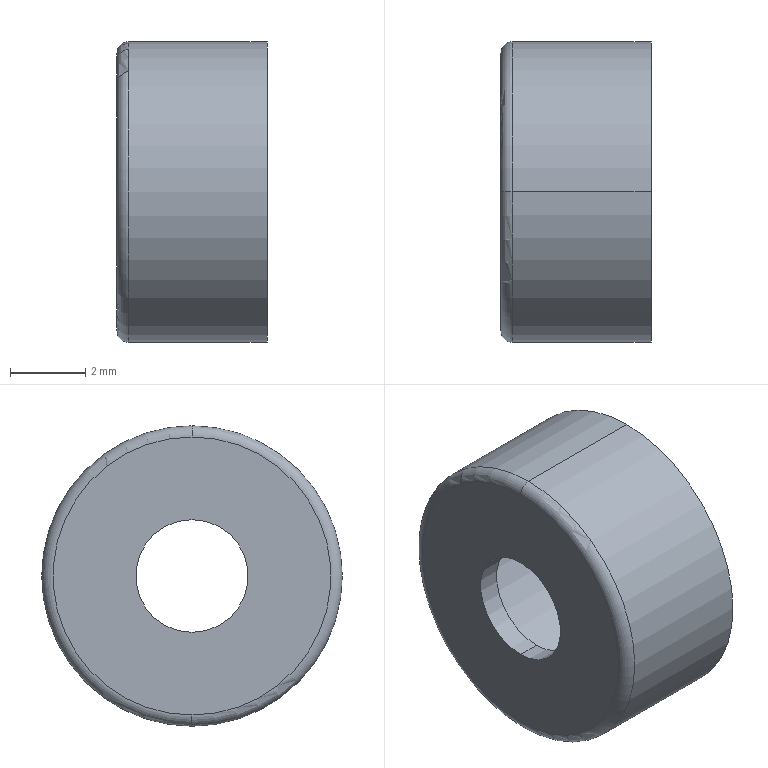Part | STEP file | 11-FG99-HXCC8b-V3.0-kkkkkk-998.11 | 1 solid | 11 faces | box 4 x 8 x 8 mm | volume 72.866 mm3 | cylinder 6 | plane 3 | torus 2 | commonest cylinder face diameters 3 x2 6.8 x2 8 x2
STEP:
#1=CARTESIAN_POINT('',(4.,0.,4.));
#2=VERTEX_POINT('',#1);
#3=CARTESIAN_POINT('',(4.,0.,-4.));
#4=VERTEX_POINT('',#3);
#5=CARTESIAN_POINT('',(4.,0.,0.));
#6=DIRECTION('',(-1.,0.,0.));
#7=DIRECTION('',(0.,0.,1.));
#8=AXIS2_PLACEMENT_3D('',#5,#6,#7);
#9=CIRCLE('',#8,4.);
#10=EDGE_CURVE('',#2,#4,#9,.T.);
#11=ORIENTED_EDGE('',*,*,#10,.T.);
#12=CARTESIAN_POINT('',(0.3,0.,-4.));
#13=VERTEX_POINT('',#12);
#14=CARTESIAN_POINT('',(4.,0.,-4.));
#15=DIRECTION('',(-1.,0.,0.));
#16=VECTOR('',#15,1000.);
#17=LINE('',#14,#16);
#18=EDGE_CURVE('',#4,#13,#17,.T.);
#19=ORIENTED_EDGE('',*,*,#18,.T.);
#20=CARTESIAN_POINT('',(0.3,0.,4.));
#21=VERTEX_POINT('',#20);
#22=CARTESIAN_POINT('',(0.3,0.,0.));
#23=DIRECTION('',(-1.,0.,0.));
#24=DIRECTION('',(0.,0.,1.));
#25=AXIS2_PLACEMENT_3D('',#22,#23,#24);
#26=CIRCLE('',#25,4.);
#27=EDGE_CURVE('',#21,#13,#26,.T.);
#28=ORIENTED_EDGE('',*,*,#27,.F.);
#29=CARTESIAN_POINT('',(4.,0.,4.));
#30=DIRECTION('',(-1.,0.,0.));
#31=VECTOR('',#30,1000.);
#32=LINE('',#29,#31);
#33=EDGE_CURVE('',#2,#21,#32,.T.);
#34=ORIENTED_EDGE('',*,*,#33,.F.);
#35=EDGE_LOOP('',(#11,#19,#28,#34));
#36=FACE_OUTER_BOUND('',#35,.T.);
#37=CARTESIAN_POINT('',(4.,0.,0.));
#38=DIRECTION('',(-1.,0.,0.));
#39=DIRECTION('',(0.,0.,1.));
#40=AXIS2_PLACEMENT_3D('',#37,#38,#39);
#41=CYLINDRICAL_SURFACE('',#40,4.);
#42=ADVANCED_FACE('',(#36),#41,.T.);
#43=CARTESIAN_POINT('',(4.,0.,-3.4));
#44=VERTEX_POINT('',#43);
#45=CARTESIAN_POINT('',(4.,0.,3.4));
#46=VERTEX_POINT('',#45);
#47=CARTESIAN_POINT('',(4.,0.,0.));
#48=DIRECTION('',(-1.,0.,0.));
#49=DIRECTION('',(0.,0.,1.));
#50=AXIS2_PLACEMENT_3D('',#47,#48,#49);
#51=CIRCLE('',#50,3.4);
#52=EDGE_CURVE('',#44,#46,#51,.T.);
#53=ORIENTED_EDGE('',*,*,#52,.F.);
#54=CARTESIAN_POINT('',(0.6,0.,-3.4));
#55=VERTEX_POINT('',#54);
#56=CARTESIAN_POINT('',(4.,0.,-3.4));
#57=DIRECTION('',(-1.,0.,0.));
#58=VECTOR('',#57,1000.);
#59=LINE('',#56,#58);
#60=EDGE_CURVE('',#44,#55,#59,.T.);
#61=ORIENTED_EDGE('',*,*,#60,.T.);
#62=CARTESIAN_POINT('',(0.6,0.,3.4));
#63=VERTEX_POINT('',#62);
#64=CARTESIAN_POINT('',(0.6,0.,0.));
#65=DIRECTION('',(-1.,0.,0.));
#66=DIRECTION('',(0.,0.,1.));
#67=AXIS2_PLACEMENT_3D('',#64,#65,#66);
#68=CIRCLE('',#67,3.4);
#69=EDGE_CURVE('',#55,#63,#68,.T.);
#70=ORIENTED_EDGE('',*,*,#69,.T.);
#71=CARTESIAN_POINT('',(4.,0.,3.4));
#72=DIRECTION('',(-1.,0.,0.));
#73=VECTOR('',#72,1000.);
#74=LINE('',#71,#73);
#75=EDGE_CURVE('',#46,#63,#74,.T.);
#76=ORIENTED_EDGE('',*,*,#75,.F.);
#77=EDGE_LOOP('',(#53,#61,#70,#76));
#78=FACE_OUTER_BOUND('',#77,.T.);
#79=CARTESIAN_POINT('',(4.,0.,0.));
#80=DIRECTION('',(-1.,0.,0.));
#81=DIRECTION('',(0.,0.,1.));
#82=AXIS2_PLACEMENT_3D('',#79,#80,#81);
#83=CYLINDRICAL_SURFACE('',#82,3.4);
#84=ADVANCED_FACE('',(#78),#83,.F.);
#85=CARTESIAN_POINT('',(0.6,0.,-1.5));
#86=VERTEX_POINT('',#85);
#87=CARTESIAN_POINT('',(0.6,0.,1.5));
#88=VERTEX_POINT('',#87);
#89=CARTESIAN_POINT('',(0.6,0.,0.));
#90=DIRECTION('',(-1.,0.,0.));
#91=DIRECTION('',(0.,0.,1.));
#92=AXIS2_PLACEMENT_3D('',#89,#90,#91);
#93=CIRCLE('',#92,1.5);
#94=EDGE_CURVE('',#86,#88,#93,.T.);
#95=ORIENTED_EDGE('',*,*,#94,.F.);
#96=CARTESIAN_POINT('',(0.,0.,-1.5));
#97=VERTEX_POINT('',#96);
#98=CARTESIAN_POINT('',(4.,0.,-1.5));
#99=DIRECTION('',(-1.,0.,0.));
#100=VECTOR('',#99,1000.);
#101=LINE('',#98,#100);
#102=EDGE_CURVE('',#86,#97,#101,.T.);
#103=ORIENTED_EDGE('',*,*,#102,.T.);
#104=CARTESIAN_POINT('',(0.,0.,1.5));
#105=VERTEX_POINT('',#104);
#106=CARTESIAN_POINT('',(0.,0.,0.));
#107=DIRECTION('',(-1.,0.,0.));
#108=DIRECTION('',(0.,0.,1.));
#109=AXIS2_PLACEMENT_3D('',#106,#107,#108);
#110=CIRCLE('',#109,1.5);
#111=EDGE_CURVE('',#97,#105,#110,.T.);
#112=ORIENTED_EDGE('',*,*,#111,.T.);
#113=CARTESIAN_POINT('',(4.,0.,1.5));
#114=DIRECTION('',(-1.,0.,0.));
#115=VECTOR('',#114,1000.);
#116=LINE('',#113,#115);
#117=EDGE_CURVE('',#88,#105,#116,.T.);
#118=ORIENTED_EDGE('',*,*,#117,.F.);
#119=EDGE_LOOP('',(#95,#103,#112,#118));
#120=FACE_OUTER_BOUND('',#119,.T.);
#121=CARTESIAN_POINT('',(4.,0.,0.));
#122=DIRECTION('',(-1.,0.,0.));
#123=DIRECTION('',(0.,0.,1.));
#124=AXIS2_PLACEMENT_3D('',#121,#122,#123);
#125=CYLINDRICAL_SURFACE('',#124,1.5);
#126=ADVANCED_FACE('',(#120),#125,.F.);
#127=ORIENTED_EDGE('',*,*,#27,.T.);
#128=CARTESIAN_POINT('',(0.,0.,-3.7));
#129=VERTEX_POINT('',#128);
#130=CARTESIAN_POINT('',(0.3,0.,-3.7));
#131=DIRECTION('',(0.,1.,0.));
#132=DIRECTION('',(0.,0.,1.));
#133=AXIS2_PLACEMENT_3D('',#130,#131,#132);
#134=CIRCLE('',#133,0.3);
#135=EDGE_CURVE('',#13,#129,#134,.T.);
#136=ORIENTED_EDGE('',*,*,#135,.T.);
#137=CARTESIAN_POINT('',(0.,0.,3.7));
#138=VERTEX_POINT('',#137);
#139=CARTESIAN_POINT('',(0.,0.,0.));
#140=DIRECTION('',(-1.,0.,0.));
#141=DIRECTION('',(0.,0.,1.));
#142=AXIS2_PLACEMENT_3D('',#139,#140,#141);
#143=CIRCLE('',#142,3.7);
#144=EDGE_CURVE('',#138,#129,#143,.T.);
#145=ORIENTED_EDGE('',*,*,#144,.F.);
#146=CARTESIAN_POINT('',(0.3,0.,3.7));
#147=DIRECTION('',(0.,-1.,0.));
#148=DIRECTION('',(0.,0.,-1.));
#149=AXIS2_PLACEMENT_3D('',#146,#147,#148);
#150=CIRCLE('',#149,0.3);
#151=EDGE_CURVE('',#21,#138,#150,.T.);
#152=ORIENTED_EDGE('',*,*,#151,.F.);
#153=EDGE_LOOP('',(#127,#136,#145,#152));
#154=FACE_OUTER_BOUND('',#153,.T.);
#155=CARTESIAN_POINT('',(0.3,0.,0.));
#156=DIRECTION('',(-1.,0.,0.));
#157=DIRECTION('',(0.,0.,1.));
#158=AXIS2_PLACEMENT_3D('',#155,#156,#157);
#159=TOROIDAL_SURFACE('',#158,3.7,0.3);
#160=ADVANCED_FACE('',(#154),#159,.T.);
#161=ORIENTED_EDGE('',*,*,#135,.F.);
#162=CARTESIAN_POINT('',(0.3,0.,0.));
#163=DIRECTION('',(-1.,0.,0.));
#164=DIRECTION('',(0.,0.,1.));
#165=AXIS2_PLACEMENT_3D('',#162,#163,#164);
#166=CIRCLE('',#165,4.);
#167=EDGE_CURVE('',#13,#21,#166,.T.);
#168=ORIENTED_EDGE('',*,*,#167,.T.);
#169=ORIENTED_EDGE('',*,*,#151,.T.);
#170=CARTESIAN_POINT('',(0.,0.,0.));
#171=DIRECTION('',(-1.,0.,0.));
#172=DIRECTION('',(0.,0.,1.));
#173=AXIS2_PLACEMENT_3D('',#170,#171,#172);
#174=CIRCLE('',#173,3.7);
#175=EDGE_CURVE('',#129,#138,#174,.T.);
#176=ORIENTED_EDGE('',*,*,#175,.F.);
#177=EDGE_LOOP('',(#161,#168,#169,#176));
#178=FACE_OUTER_BOUND('',#177,.T.);
#179=CARTESIAN_POINT('',(0.3,0.,0.));
#180=DIRECTION('',(-1.,0.,0.));
#181=DIRECTION('',(0.,0.,1.));
#182=AXIS2_PLACEMENT_3D('',#179,#180,#181);
#183=TOROIDAL_SURFACE('',#182,3.7,0.3);
#184=ADVANCED_FACE('',(#178),#183,.T.);
#185=CARTESIAN_POINT('',(0.,0.,0.));
#186=DIRECTION('',(-1.,0.,0.));
#187=DIRECTION('',(0.,0.,1.));
#188=AXIS2_PLACEMENT_3D('',#185,#186,#187);
#189=CIRCLE('',#188,1.5);
#190=EDGE_CURVE('',#105,#97,#189,.T.);
#191=ORIENTED_EDGE('',*,*,#190,.F.);
#192=ORIENTED_EDGE('',*,*,#111,.F.);
#193=EDGE_LOOP('',(#191,#192));
#194=FACE_BOUND('',#193,.T.);
#195=ORIENTED_EDGE('',*,*,#144,.T.);
#196=ORIENTED_EDGE('',*,*,#175,.T.);
#197=EDGE_LOOP('',(#195,#196));
#198=FACE_OUTER_BOUND('',#197,.T.);
#199=CARTESIAN_POINT('',(0.,3.7,0.));
#200=DIRECTION('',(1.,0.,0.));
#201=DIRECTION('',(0.,0.,-1.));
#202=AXIS2_PLACEMENT_3D('',#199,#200,#201);
#203=PLANE('',#202);
#204=ADVANCED_FACE('',(#194,#198),#203,.F.);
#205=ORIENTED_EDGE('',*,*,#102,.F.);
#206=CARTESIAN_POINT('',(0.6,0.,0.));
#207=DIRECTION('',(-1.,0.,0.));
#208=DIRECTION('',(0.,0.,1.));
#209=AXIS2_PLACEMENT_3D('',#206,#207,#208);
#210=CIRCLE('',#209,1.5);
#211=EDGE_CURVE('',#88,#86,#210,.T.);
#212=ORIENTED_EDGE('',*,*,#211,.F.);
#213=ORIENTED_EDGE('',*,*,#117,.T.);
#214=ORIENTED_EDGE('',*,*,#190,.T.);
#215=EDGE_LOOP('',(#205,#212,#213,#214));
#216=FACE_OUTER_BOUND('',#215,.T.);
#217=CARTESIAN_POINT('',(4.,0.,0.));
#218=DIRECTION('',(-1.,0.,0.));
#219=DIRECTION('',(0.,0.,1.));
#220=AXIS2_PLACEMENT_3D('',#217,#218,#219);
#221=CYLINDRICAL_SURFACE('',#220,1.5);
#222=ADVANCED_FACE('',(#216),#221,.F.);
#223=CARTESIAN_POINT('',(0.6,0.,0.));
#224=DIRECTION('',(-1.,0.,0.));
#225=DIRECTION('',(0.,0.,1.));
#226=AXIS2_PLACEMENT_3D('',#223,#224,#225);
#227=CIRCLE('',#226,3.4);
#228=EDGE_CURVE('',#63,#55,#227,.T.);
#229=ORIENTED_EDGE('',*,*,#228,.F.);
#230=ORIENTED_EDGE('',*,*,#69,.F.);
#231=EDGE_LOOP('',(#229,#230));
#232=FACE_OUTER_BOUND('',#231,.T.);
#233=ORIENTED_EDGE('',*,*,#211,.T.);
#234=ORIENTED_EDGE('',*,*,#94,.T.);
#235=EDGE_LOOP('',(#233,#234));
#236=FACE_BOUND('',#235,.T.);
#237=CARTESIAN_POINT('',(0.6,1.5,0.));
#238=DIRECTION('',(-1.,0.,0.));
#239=DIRECTION('',(0.,0.,1.));
#240=AXIS2_PLACEMENT_3D('',#237,#238,#239);
#241=PLANE('',#240);
#242=ADVANCED_FACE('',(#232,#236),#241,.F.);
#243=ORIENTED_EDGE('',*,*,#60,.F.);
#244=CARTESIAN_POINT('',(4.,0.,0.));
#245=DIRECTION('',(-1.,0.,0.));
#246=DIRECTION('',(0.,0.,1.));
#247=AXIS2_PLACEMENT_3D('',#244,#245,#246);
#248=CIRCLE('',#247,3.4);
#249=EDGE_CURVE('',#46,#44,#248,.T.);
#250=ORIENTED_EDGE('',*,*,#249,.F.);
#251=ORIENTED_EDGE('',*,*,#75,.T.);
#252=ORIENTED_EDGE('',*,*,#228,.T.);
#253=EDGE_LOOP('',(#243,#250,#251,#252));
#254=FACE_OUTER_BOUND('',#253,.T.);
#255=CARTESIAN_POINT('',(4.,0.,0.));
#256=DIRECTION('',(-1.,0.,0.));
#257=DIRECTION('',(0.,0.,1.));
#258=AXIS2_PLACEMENT_3D('',#255,#256,#257);
#259=CYLINDRICAL_SURFACE('',#258,3.4);
#260=ADVANCED_FACE('',(#254),#259,.F.);
#261=ORIENTED_EDGE('',*,*,#10,.F.);
#262=CARTESIAN_POINT('',(4.,0.,0.));
#263=DIRECTION('',(-1.,0.,0.));
#264=DIRECTION('',(0.,0.,1.));
#265=AXIS2_PLACEMENT_3D('',#262,#263,#264);
#266=CIRCLE('',#265,4.);
#267=EDGE_CURVE('',#4,#2,#266,.T.);
#268=ORIENTED_EDGE('',*,*,#267,.F.);
#269=EDGE_LOOP('',(#261,#268));
#270=FACE_OUTER_BOUND('',#269,.T.);
#271=ORIENTED_EDGE('',*,*,#249,.T.);
#272=ORIENTED_EDGE('',*,*,#52,.T.);
#273=EDGE_LOOP('',(#271,#272));
#274=FACE_BOUND('',#273,.T.);
#275=CARTESIAN_POINT('',(4.,3.4,0.));
#276=DIRECTION('',(-1.,0.,0.));
#277=DIRECTION('',(0.,0.,1.));
#278=AXIS2_PLACEMENT_3D('',#275,#276,#277);
#279=PLANE('',#278);
#280=ADVANCED_FACE('',(#270,#274),#279,.F.);
#281=ORIENTED_EDGE('',*,*,#18,.F.);
#282=ORIENTED_EDGE('',*,*,#267,.T.);
#283=ORIENTED_EDGE('',*,*,#33,.T.);
#284=ORIENTED_EDGE('',*,*,#167,.F.);
#285=EDGE_LOOP('',(#281,#282,#283,#284));
#286=FACE_OUTER_BOUND('',#285,.T.);
#287=CARTESIAN_POINT('',(4.,0.,0.));
#288=DIRECTION('',(-1.,0.,0.));
#289=DIRECTION('',(0.,0.,1.));
#290=AXIS2_PLACEMENT_3D('',#287,#288,#289);
#291=CYLINDRICAL_SURFACE('',#290,4.);
#292=ADVANCED_FACE('',(#286),#291,.T.);
#293=CLOSED_SHELL('',(#42,#84,#126,#160,#184,#204,#222,#242,#260,#280,#292));
#294=MANIFOLD_SOLID_BREP('',#293);
#295=CARTESIAN_POINT('',(0.,0.,0.));
#296=DIRECTION('',(0.,0.,1.));
#297=DIRECTION('',(1.,0.,0.));
#298=AXIS2_PLACEMENT_3D('',#295,#296,#297);
#299=(LENGTH_UNIT()NAMED_UNIT(*)SI_UNIT(.MILLI.,.METRE.));
#300=UNCERTAINTY_MEASURE_WITH_UNIT(LENGTH_MEASURE(0.00001),#299,'','');
#301=(NAMED_UNIT(*)PLANE_ANGLE_UNIT()SI_UNIT($,.RADIAN.));
#302=(NAMED_UNIT(*)SI_UNIT($,.STERADIAN.)SOLID_ANGLE_UNIT());
#303=(GEOMETRIC_REPRESENTATION_CONTEXT(3)GLOBAL_UNCERTAINTY_ASSIGNED_CONTEXT((#300))GLOBAL_UNIT_ASSIGNED_CONTEXT((#299,#301,#302))REPRESENTATION_CONTEXT('',''));
#304=ADVANCED_BREP_SHAPE_REPRESENTATION('',(#294,#298),#303);